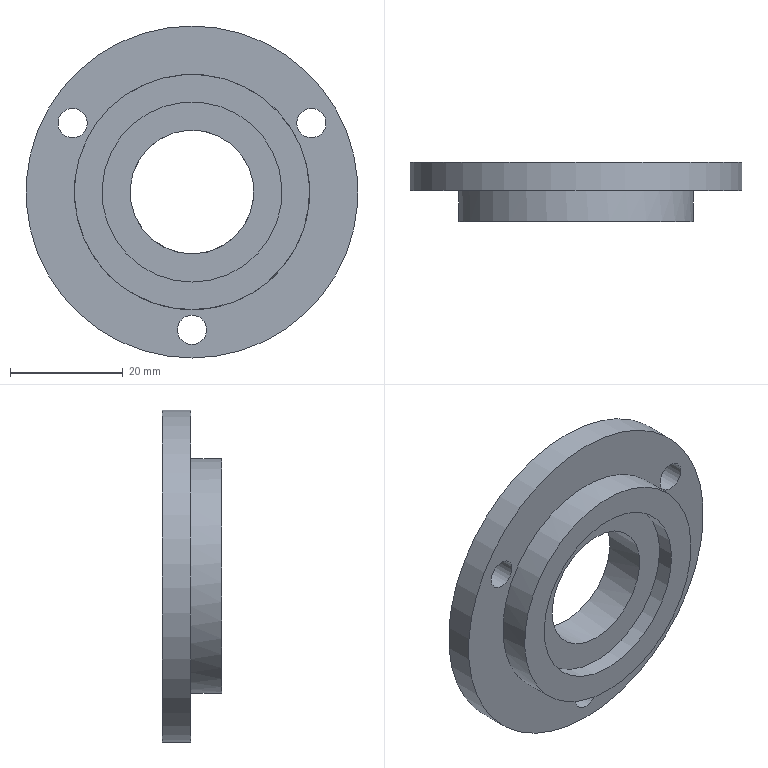Part | STEP file | 冲床-300配套压波_id630_x_t | 1 solid | 11 faces | box 59 x 10.5 x 59 mm | volume 15635 mm3 | cylinder 7 | plane 4 | commonest cylinder face diameters 5.2 x3 22 x1 32 x1 41.8 x1 59 x1
STEP:
#1=CARTESIAN_POINT('',(1235.221,105.,187.129));
#2=VERTEX_POINT('',#1);
#3=CARTESIAN_POINT('',(1250.,105.,172.35));
#4=DIRECTION('',(0.,-1.,0.));
#5=DIRECTION('',(-0.7071,0.,0.7071));
#6=AXIS2_PLACEMENT_3D('',#3,#4,#5);
#7=CIRCLE('',#6,20.9);
#8=EDGE_CURVE('',#2,#2,#7,.T.);
#9=ORIENTED_EDGE('',*,*,#8,.T.);
#10=EDGE_LOOP('',(#9));
#11=FACE_BOUND('',#10,.T.);
#12=CARTESIAN_POINT('',(1250.,99.5,151.45));
#13=VERTEX_POINT('',#12);
#14=CARTESIAN_POINT('',(1250.,99.5,172.35));
#15=DIRECTION('',(0.,1.,0.));
#16=DIRECTION('',(0.,0.,-1.));
#17=AXIS2_PLACEMENT_3D('',#14,#15,#16);
#18=CIRCLE('',#17,20.9);
#19=EDGE_CURVE('',#13,#13,#18,.T.);
#20=ORIENTED_EDGE('',*,*,#19,.T.);
#21=EDGE_LOOP('',(#20));
#22=FACE_BOUND('',#21,.T.);
#23=CARTESIAN_POINT('',(1250.,100.,172.35));
#24=DIRECTION('',(0.,1.,0.));
#25=DIRECTION('',(-0.7071,0.,0.7071));
#26=AXIS2_PLACEMENT_3D('',#23,#24,#25);
#27=CYLINDRICAL_SURFACE('',#26,20.9);
#28=ADVANCED_FACE('',(#11,#22),#27,.T.);
#29=CARTESIAN_POINT('',(1250.,110.,201.85));
#30=VERTEX_POINT('',#29);
#31=CARTESIAN_POINT('',(1250.,110.,172.35));
#32=DIRECTION('',(0.,1.,0.));
#33=DIRECTION('',(0.,0.,1.));
#34=AXIS2_PLACEMENT_3D('',#31,#32,#33);
#35=CIRCLE('',#34,29.5);
#36=EDGE_CURVE('',#30,#30,#35,.T.);
#37=ORIENTED_EDGE('',*,*,#36,.F.);
#38=EDGE_LOOP('',(#37));
#39=FACE_BOUND('',#38,.T.);
#40=CARTESIAN_POINT('',(1250.,105.,201.85));
#41=VERTEX_POINT('',#40);
#42=CARTESIAN_POINT('',(1250.,105.,172.35));
#43=DIRECTION('',(0.,1.,0.));
#44=DIRECTION('',(0.,0.,1.));
#45=AXIS2_PLACEMENT_3D('',#42,#43,#44);
#46=CIRCLE('',#45,29.5);
#47=EDGE_CURVE('',#41,#41,#46,.T.);
#48=ORIENTED_EDGE('',*,*,#47,.T.);
#49=EDGE_LOOP('',(#48));
#50=FACE_BOUND('',#49,.T.);
#51=CARTESIAN_POINT('',(1250.,110.,172.35));
#52=DIRECTION('',(0.,-1.,0.));
#53=DIRECTION('',(0.7071,0.,-0.7071));
#54=AXIS2_PLACEMENT_3D('',#51,#52,#53);
#55=CYLINDRICAL_SURFACE('',#54,29.5);
#56=ADVANCED_FACE('',(#39,#50),#55,.T.);
#57=CARTESIAN_POINT('',(1271.218,110.,187.2));
#58=VERTEX_POINT('',#57);
#59=CARTESIAN_POINT('',(1271.218,110.,184.6));
#60=DIRECTION('',(0.,1.,0.));
#61=DIRECTION('',(0.,0.,1.));
#62=AXIS2_PLACEMENT_3D('',#59,#60,#61);
#63=CIRCLE('',#62,2.6);
#64=EDGE_CURVE('',#58,#58,#63,.T.);
#65=ORIENTED_EDGE('',*,*,#64,.F.);
#66=EDGE_LOOP('',(#65));
#67=FACE_BOUND('',#66,.T.);
#68=CARTESIAN_POINT('',(1250.,110.,150.45));
#69=VERTEX_POINT('',#68);
#70=CARTESIAN_POINT('',(1250.,110.,147.85));
#71=DIRECTION('',(0.,1.,0.));
#72=DIRECTION('',(0.,0.,1.));
#73=AXIS2_PLACEMENT_3D('',#70,#71,#72);
#74=CIRCLE('',#73,2.6);
#75=EDGE_CURVE('',#69,#69,#74,.T.);
#76=ORIENTED_EDGE('',*,*,#75,.F.);
#77=EDGE_LOOP('',(#76));
#78=FACE_BOUND('',#77,.T.);
#79=CARTESIAN_POINT('',(1228.782,110.,187.2));
#80=VERTEX_POINT('',#79);
#81=CARTESIAN_POINT('',(1228.782,110.,184.6));
#82=DIRECTION('',(0.,1.,0.));
#83=DIRECTION('',(0.,0.,1.));
#84=AXIS2_PLACEMENT_3D('',#81,#82,#83);
#85=CIRCLE('',#84,2.6);
#86=EDGE_CURVE('',#80,#80,#85,.T.);
#87=ORIENTED_EDGE('',*,*,#86,.F.);
#88=EDGE_LOOP('',(#87));
#89=FACE_BOUND('',#88,.T.);
#90=ORIENTED_EDGE('',*,*,#36,.T.);
#91=EDGE_LOOP('',(#90));
#92=FACE_BOUND('',#91,.T.);
#93=CARTESIAN_POINT('',(1242.222,110.,180.128));
#94=VERTEX_POINT('',#93);
#95=CARTESIAN_POINT('',(1250.,110.,172.35));
#96=DIRECTION('',(0.,-1.,0.));
#97=DIRECTION('',(-0.7071,0.,0.7071));
#98=AXIS2_PLACEMENT_3D('',#95,#96,#97);
#99=CIRCLE('',#98,11.);
#100=EDGE_CURVE('',#94,#94,#99,.T.);
#101=ORIENTED_EDGE('',*,*,#100,.T.);
#102=EDGE_LOOP('',(#101));
#103=FACE_BOUND('',#102,.T.);
#104=CARTESIAN_POINT('',(1250.,110.,172.35));
#105=DIRECTION('',(0.,-1.,0.));
#106=DIRECTION('',(0.7071,0.,-0.7071));
#107=AXIS2_PLACEMENT_3D('',#104,#105,#106);
#108=PLANE('',#107);
#109=ADVANCED_FACE('',(#67,#78,#89,#92,#103),#108,.F.);
#110=CARTESIAN_POINT('',(1271.218,105.,187.2));
#111=VERTEX_POINT('',#110);
#112=CARTESIAN_POINT('',(1271.218,105.,184.6));
#113=DIRECTION('',(0.,1.,0.));
#114=DIRECTION('',(0.,0.,1.));
#115=AXIS2_PLACEMENT_3D('',#112,#113,#114);
#116=CIRCLE('',#115,2.6);
#117=EDGE_CURVE('',#111,#111,#116,.T.);
#118=ORIENTED_EDGE('',*,*,#117,.T.);
#119=EDGE_LOOP('',(#118));
#120=FACE_BOUND('',#119,.T.);
#121=CARTESIAN_POINT('',(1250.,105.,150.45));
#122=VERTEX_POINT('',#121);
#123=CARTESIAN_POINT('',(1250.,105.,147.85));
#124=DIRECTION('',(0.,1.,0.));
#125=DIRECTION('',(0.,0.,1.));
#126=AXIS2_PLACEMENT_3D('',#123,#124,#125);
#127=CIRCLE('',#126,2.6);
#128=EDGE_CURVE('',#122,#122,#127,.T.);
#129=ORIENTED_EDGE('',*,*,#128,.T.);
#130=EDGE_LOOP('',(#129));
#131=FACE_BOUND('',#130,.T.);
#132=CARTESIAN_POINT('',(1228.782,105.,187.2));
#133=VERTEX_POINT('',#132);
#134=CARTESIAN_POINT('',(1228.782,105.,184.6));
#135=DIRECTION('',(0.,1.,0.));
#136=DIRECTION('',(0.,0.,1.));
#137=AXIS2_PLACEMENT_3D('',#134,#135,#136);
#138=CIRCLE('',#137,2.6);
#139=EDGE_CURVE('',#133,#133,#138,.T.);
#140=ORIENTED_EDGE('',*,*,#139,.T.);
#141=EDGE_LOOP('',(#140));
#142=FACE_BOUND('',#141,.T.);
#143=ORIENTED_EDGE('',*,*,#47,.F.);
#144=EDGE_LOOP('',(#143));
#145=FACE_BOUND('',#144,.T.);
#146=ORIENTED_EDGE('',*,*,#8,.F.);
#147=EDGE_LOOP('',(#146));
#148=FACE_BOUND('',#147,.T.);
#149=CARTESIAN_POINT('',(1250.,105.,172.35));
#150=DIRECTION('',(0.,-1.,0.));
#151=DIRECTION('',(0.7071,0.,-0.7071));
#152=AXIS2_PLACEMENT_3D('',#149,#150,#151);
#153=PLANE('',#152);
#154=ADVANCED_FACE('',(#120,#131,#142,#145,#148),#153,.T.);
#155=CARTESIAN_POINT('',(1250.,99.5,156.35));
#156=VERTEX_POINT('',#155);
#157=CARTESIAN_POINT('',(1250.,99.5,172.35));
#158=DIRECTION('',(0.,1.,0.));
#159=DIRECTION('',(0.,0.,-1.));
#160=AXIS2_PLACEMENT_3D('',#157,#158,#159);
#161=CIRCLE('',#160,16.);
#162=EDGE_CURVE('',#156,#156,#161,.T.);
#163=ORIENTED_EDGE('',*,*,#162,.T.);
#164=EDGE_LOOP('',(#163));
#165=FACE_BOUND('',#164,.T.);
#166=ORIENTED_EDGE('',*,*,#19,.F.);
#167=EDGE_LOOP('',(#166));
#168=FACE_BOUND('',#167,.T.);
#169=CARTESIAN_POINT('',(1250.,99.5,162.35));
#170=DIRECTION('',(0.,1.,0.));
#171=DIRECTION('',(0.,0.,1.));
#172=AXIS2_PLACEMENT_3D('',#169,#170,#171);
#173=PLANE('',#172);
#174=ADVANCED_FACE('',(#165,#168),#173,.F.);
#175=CARTESIAN_POINT('',(1250.,102.5,161.35));
#176=VERTEX_POINT('',#175);
#177=CARTESIAN_POINT('',(1250.,102.5,172.35));
#178=DIRECTION('',(0.,-1.,0.));
#179=DIRECTION('',(0.,0.,-1.));
#180=AXIS2_PLACEMENT_3D('',#177,#178,#179);
#181=CIRCLE('',#180,11.);
#182=EDGE_CURVE('',#176,#176,#181,.T.);
#183=ORIENTED_EDGE('',*,*,#182,.T.);
#184=EDGE_LOOP('',(#183));
#185=FACE_BOUND('',#184,.T.);
#186=ORIENTED_EDGE('',*,*,#100,.F.);
#187=EDGE_LOOP('',(#186));
#188=FACE_BOUND('',#187,.T.);
#189=CARTESIAN_POINT('',(1250.,100.,172.35));
#190=DIRECTION('',(0.,1.,0.));
#191=DIRECTION('',(-0.7071,0.,0.7071));
#192=AXIS2_PLACEMENT_3D('',#189,#190,#191);
#193=CYLINDRICAL_SURFACE('',#192,11.);
#194=ADVANCED_FACE('',(#185,#188),#193,.F.);
#195=CARTESIAN_POINT('',(1250.,102.5,156.35));
#196=VERTEX_POINT('',#195);
#197=CARTESIAN_POINT('',(1250.,102.5,172.35));
#198=DIRECTION('',(0.,1.,0.));
#199=DIRECTION('',(0.,0.,-1.));
#200=AXIS2_PLACEMENT_3D('',#197,#198,#199);
#201=CIRCLE('',#200,16.);
#202=EDGE_CURVE('',#196,#196,#201,.T.);
#203=ORIENTED_EDGE('',*,*,#202,.F.);
#204=EDGE_LOOP('',(#203));
#205=FACE_BOUND('',#204,.T.);
#206=ORIENTED_EDGE('',*,*,#182,.F.);
#207=EDGE_LOOP('',(#206));
#208=FACE_BOUND('',#207,.T.);
#209=CARTESIAN_POINT('',(1250.,102.5,172.35));
#210=DIRECTION('',(0.,1.,0.));
#211=DIRECTION('',(0.,0.,-1.));
#212=AXIS2_PLACEMENT_3D('',#209,#210,#211);
#213=PLANE('',#212);
#214=ADVANCED_FACE('',(#205,#208),#213,.F.);
#215=ORIENTED_EDGE('',*,*,#202,.T.);
#216=EDGE_LOOP('',(#215));
#217=FACE_BOUND('',#216,.T.);
#218=ORIENTED_EDGE('',*,*,#162,.F.);
#219=EDGE_LOOP('',(#218));
#220=FACE_BOUND('',#219,.T.);
#221=CARTESIAN_POINT('',(1250.,99.5,172.35));
#222=DIRECTION('',(0.,1.,0.));
#223=DIRECTION('',(-1.,0.,0.));
#224=AXIS2_PLACEMENT_3D('',#221,#222,#223);
#225=CYLINDRICAL_SURFACE('',#224,16.);
#226=ADVANCED_FACE('',(#217,#220),#225,.F.);
#227=ORIENTED_EDGE('',*,*,#139,.F.);
#228=EDGE_LOOP('',(#227));
#229=FACE_BOUND('',#228,.T.);
#230=ORIENTED_EDGE('',*,*,#86,.T.);
#231=EDGE_LOOP('',(#230));
#232=FACE_BOUND('',#231,.T.);
#233=CARTESIAN_POINT('',(1228.782,97.8,184.6));
#234=DIRECTION('',(0.,1.,0.));
#235=DIRECTION('',(-1.,0.,0.));
#236=AXIS2_PLACEMENT_3D('',#233,#234,#235);
#237=CYLINDRICAL_SURFACE('',#236,2.6);
#238=ADVANCED_FACE('',(#229,#232),#237,.F.);
#239=ORIENTED_EDGE('',*,*,#128,.F.);
#240=EDGE_LOOP('',(#239));
#241=FACE_BOUND('',#240,.T.);
#242=ORIENTED_EDGE('',*,*,#75,.T.);
#243=EDGE_LOOP('',(#242));
#244=FACE_BOUND('',#243,.T.);
#245=CARTESIAN_POINT('',(1250.,97.8,147.85));
#246=DIRECTION('',(0.,1.,0.));
#247=DIRECTION('',(-1.,0.,0.));
#248=AXIS2_PLACEMENT_3D('',#245,#246,#247);
#249=CYLINDRICAL_SURFACE('',#248,2.6);
#250=ADVANCED_FACE('',(#241,#244),#249,.F.);
#251=ORIENTED_EDGE('',*,*,#117,.F.);
#252=EDGE_LOOP('',(#251));
#253=FACE_BOUND('',#252,.T.);
#254=ORIENTED_EDGE('',*,*,#64,.T.);
#255=EDGE_LOOP('',(#254));
#256=FACE_BOUND('',#255,.T.);
#257=CARTESIAN_POINT('',(1271.218,97.8,184.6));
#258=DIRECTION('',(0.,1.,0.));
#259=DIRECTION('',(-1.,0.,0.));
#260=AXIS2_PLACEMENT_3D('',#257,#258,#259);
#261=CYLINDRICAL_SURFACE('',#260,2.6);
#262=ADVANCED_FACE('',(#253,#256),#261,.F.);
#263=CLOSED_SHELL('',(#28,#56,#109,#154,#174,#194,#214,#226,#238,#250,#262));
#264=MANIFOLD_SOLID_BREP('',#263);
#265=(LENGTH_UNIT()NAMED_UNIT(*)SI_UNIT(.MILLI.,.METRE.));
#266=UNCERTAINTY_MEASURE_WITH_UNIT(LENGTH_MEASURE(0.00002),#265,'','');
#267=(NAMED_UNIT(*)PLANE_ANGLE_UNIT()SI_UNIT($,.RADIAN.));
#268=PLANE_ANGLE_MEASURE_WITH_UNIT(PLANE_ANGLE_MEASURE(0.01745),#267);
#269=DIMENSIONAL_EXPONENTS(0.,0.,0.,0.,0.,0.,0.);
#270=(CONVERSION_BASED_UNIT('DEGREE',#268)NAMED_UNIT(#269)PLANE_ANGLE_UNIT());
#271=(NAMED_UNIT(*)SI_UNIT($,.STERADIAN.)SOLID_ANGLE_UNIT());
#272=(GEOMETRIC_REPRESENTATION_CONTEXT(3)GLOBAL_UNCERTAINTY_ASSIGNED_CONTEXT((#266))GLOBAL_UNIT_ASSIGNED_CONTEXT((#265,#270,#271))REPRESENTATION_CONTEXT('',''));
#273=ADVANCED_BREP_SHAPE_REPRESENTATION('',(#264),#272);